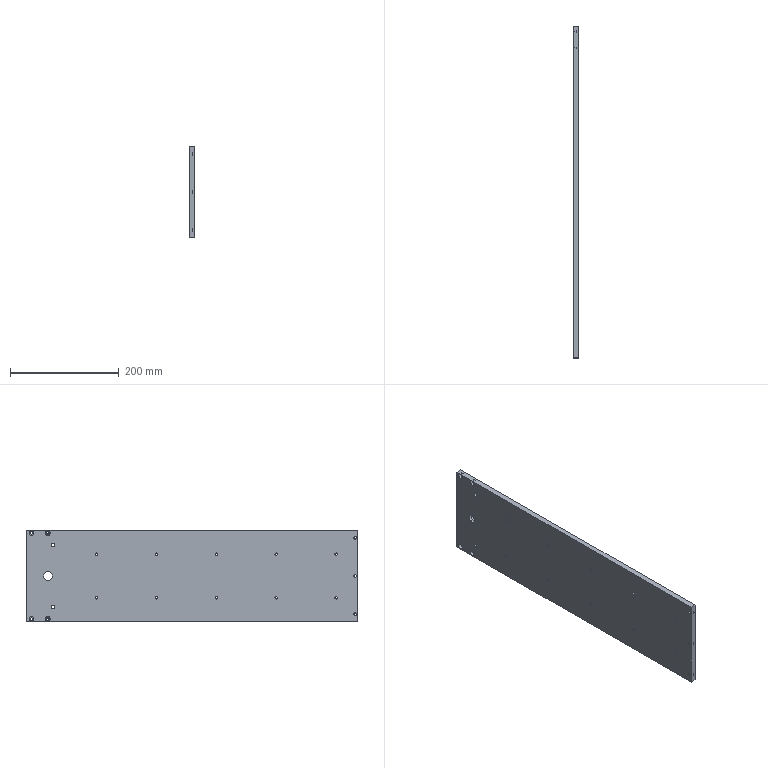Part | STEP file | 03-24 Feed mechanism support plate 2 | 1 solid | 112 faces | box 10 x 609 x 168 mm | volume 1013118 mm3 | cylinder 82 | plane 24 | cone 6 | commonest cylinder face diameters 4.5 x34 9 x34 3.3 x6 6.5 x4 16 x2 19 x2